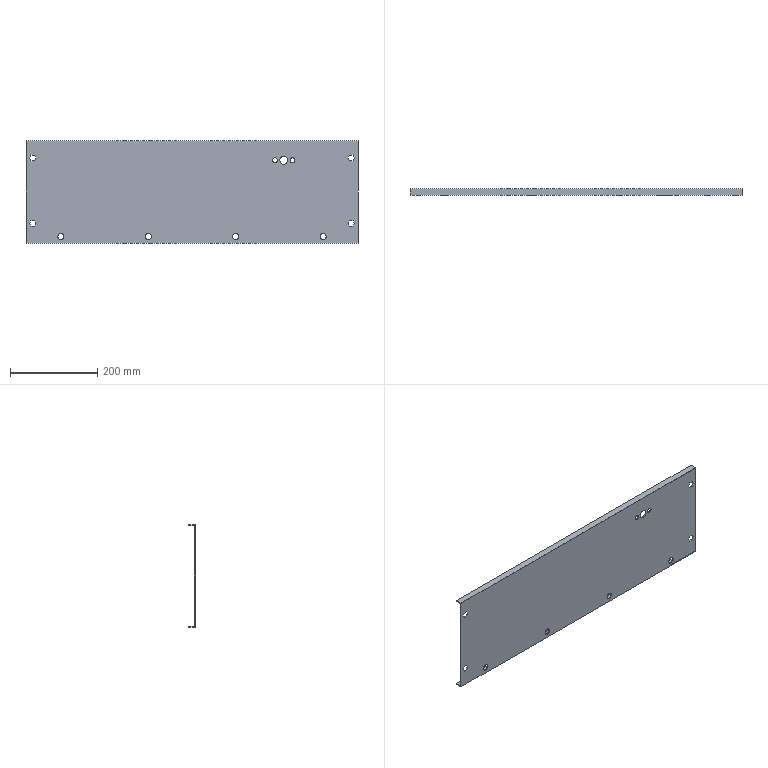Part | SolidWorks | features BaseBody 1 | 1 solid | 48 faces | box 760 x 15 x 234.5 mm | volume 392669 mm3 | plane 34 | cylinder 14 | commonest cylinder face diameters 14 x8 11 x4 18 x2